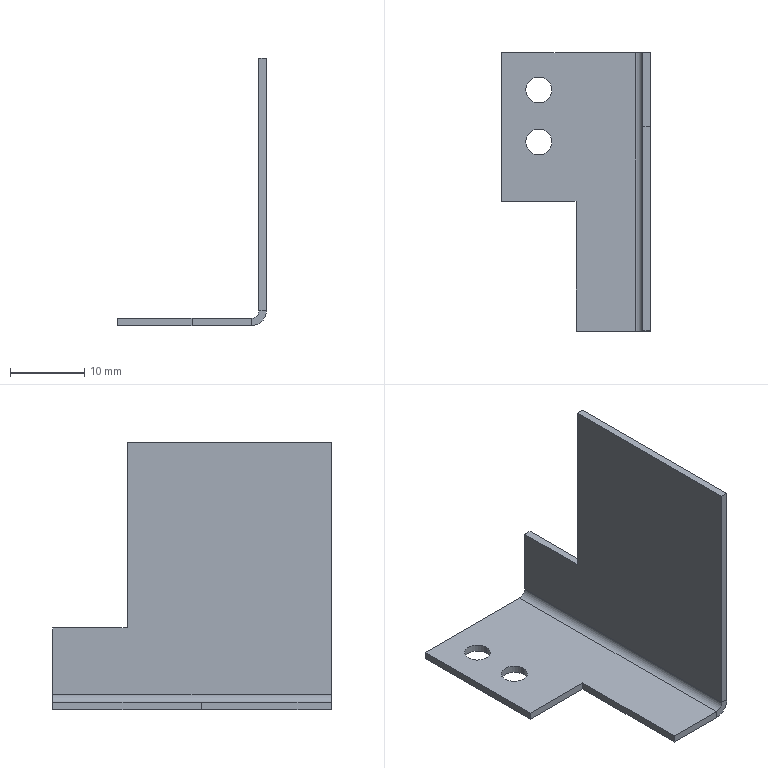Part | STEP file | Proximity switch bracket 3V1.201001 | 1 solid | 22 faces | box 20 x 37.5 x 36 mm | volume 1594 mm3 | plane 16 | cylinder 6 | commonest cylinder face diameters 3.5 x4 2 x1 4 x1
STEP:
#1=CARTESIAN_POINT('',(0.,0.,0.));
#2=DIRECTION('',(0.,0.,1.));
#3=DIRECTION('',(1.,0.,0.));
#4=AXIS2_PLACEMENT_3D('',#1,#2,#3);
#5=CARTESIAN_POINT('',(3.25,13.75,0.));
#6=VERTEX_POINT('',#5);
#7=CARTESIAN_POINT('',(3.25,13.75,-1.));
#8=VERTEX_POINT('',#7);
#9=CARTESIAN_POINT('',(3.25,13.75,0.));
#10=DIRECTION('',(0.,0.,-1.));
#11=VECTOR('',#10,1.);
#12=LINE('',#9,#11);
#13=CARTESIAN_POINT('',(5.,13.75,0.));
#14=DIRECTION('',(0.,0.,-1.));
#15=DIRECTION('',(-1.,0.,0.));
#16=AXIS2_PLACEMENT_3D('',#13,#14,#15);
#17=CYLINDRICAL_SURFACE('',#16,1.75);
#18=CARTESIAN_POINT('',(6.283,0.));
#19=DIRECTION('',(0.,1.));
#20=VECTOR('',#19,1.);
#21=LINE('',#18,#20);
#22=(GEOMETRIC_REPRESENTATION_CONTEXT(2)PARAMETRIC_REPRESENTATION_CONTEXT()REPRESENTATION_CONTEXT('',''));
#23=DEFINITIONAL_REPRESENTATION('',(#21),#22);
#24=PCURVE('',#17,#23);
#25=CARTESIAN_POINT('',(5.,13.75,0.));
#26=DIRECTION('',(0.,0.,-1.));
#27=DIRECTION('',(-1.,0.,0.));
#28=AXIS2_PLACEMENT_3D('',#25,#26,#27);
#29=CYLINDRICAL_SURFACE('',#28,1.75);
#30=CARTESIAN_POINT('',(0.,0.));
#31=DIRECTION('',(0.,1.));
#32=VECTOR('',#31,1.);
#33=LINE('',#30,#32);
#34=(GEOMETRIC_REPRESENTATION_CONTEXT(2)PARAMETRIC_REPRESENTATION_CONTEXT()REPRESENTATION_CONTEXT('',''));
#35=DEFINITIONAL_REPRESENTATION('',(#33),#34);
#36=PCURVE('',#29,#35);
#37=SURFACE_CURVE('',#12,(#24,#36),.PCURVE_S1.);
#38=EDGE_CURVE('',#6,#8,#37,.T.);
#39=ORIENTED_EDGE('',*,*,#38,.T.);
#40=CARTESIAN_POINT('',(6.75,13.75,-1.));
#41=VERTEX_POINT('',#40);
#42=CARTESIAN_POINT('',(5.,13.75,-1.));
#43=DIRECTION('',(0.,0.,-1.));
#44=DIRECTION('',(-1.,0.,0.));
#45=AXIS2_PLACEMENT_3D('',#42,#43,#44);
#46=CIRCLE('',#45,1.75);
#47=CARTESIAN_POINT('',(0.,1.));
#48=DIRECTION('',(1.,0.));
#49=VECTOR('',#48,1.);
#50=LINE('',#47,#49);
#51=(GEOMETRIC_REPRESENTATION_CONTEXT(2)PARAMETRIC_REPRESENTATION_CONTEXT()REPRESENTATION_CONTEXT('',''));
#52=DEFINITIONAL_REPRESENTATION('',(#50),#51);
#53=PCURVE('',#17,#52);
#54=CARTESIAN_POINT('',(0.,18.75,-1.));
#55=DIRECTION('',(0.,0.,-1.));
#56=DIRECTION('',(-1.,0.,0.));
#57=AXIS2_PLACEMENT_3D('',#54,#55,#56);
#58=PLANE('',#57);
#59=CARTESIAN_POINT('',(-5.,-5.));
#60=DIRECTION('',(1.,0.));
#61=AXIS2_PLACEMENT_2D('',#59,#60);
#62=CIRCLE('',#61,1.75);
#63=(GEOMETRIC_REPRESENTATION_CONTEXT(2)PARAMETRIC_REPRESENTATION_CONTEXT()REPRESENTATION_CONTEXT('',''));
#64=DEFINITIONAL_REPRESENTATION('',(#62),#63);
#65=PCURVE('',#58,#64);
#66=SURFACE_CURVE('',#46,(#53,#65),.PCURVE_S1.);
#67=EDGE_CURVE('',#41,#8,#66,.T.);
#68=ORIENTED_EDGE('',*,*,#67,.F.);
#69=CARTESIAN_POINT('',(6.75,13.75,0.));
#70=VERTEX_POINT('',#69);
#71=CARTESIAN_POINT('',(6.75,13.75,0.));
#72=DIRECTION('',(0.,0.,-1.));
#73=VECTOR('',#72,1.);
#74=LINE('',#71,#73);
#75=CARTESIAN_POINT('',(3.142,0.));
#76=DIRECTION('',(0.,1.));
#77=VECTOR('',#76,1.);
#78=LINE('',#75,#77);
#79=(GEOMETRIC_REPRESENTATION_CONTEXT(2)PARAMETRIC_REPRESENTATION_CONTEXT()REPRESENTATION_CONTEXT('',''));
#80=DEFINITIONAL_REPRESENTATION('',(#78),#79);
#81=PCURVE('',#17,#80);
#82=CARTESIAN_POINT('',(3.142,0.));
#83=DIRECTION('',(0.,1.));
#84=VECTOR('',#83,1.);
#85=LINE('',#82,#84);
#86=(GEOMETRIC_REPRESENTATION_CONTEXT(2)PARAMETRIC_REPRESENTATION_CONTEXT()REPRESENTATION_CONTEXT('',''));
#87=DEFINITIONAL_REPRESENTATION('',(#85),#86);
#88=PCURVE('',#29,#87);
#89=SURFACE_CURVE('',#74,(#81,#88),.PCURVE_S1.);
#90=EDGE_CURVE('',#70,#41,#89,.T.);
#91=ORIENTED_EDGE('',*,*,#90,.F.);
#92=CARTESIAN_POINT('',(5.,13.75,0.));
#93=DIRECTION('',(0.,0.,-1.));
#94=DIRECTION('',(-1.,0.,0.));
#95=AXIS2_PLACEMENT_3D('',#92,#93,#94);
#96=CIRCLE('',#95,1.75);
#97=CARTESIAN_POINT('',(0.,0.));
#98=DIRECTION('',(1.,0.));
#99=VECTOR('',#98,1.);
#100=LINE('',#97,#99);
#101=(GEOMETRIC_REPRESENTATION_CONTEXT(2)PARAMETRIC_REPRESENTATION_CONTEXT()REPRESENTATION_CONTEXT('',''));
#102=DEFINITIONAL_REPRESENTATION('',(#100),#101);
#103=PCURVE('',#17,#102);
#104=CARTESIAN_POINT('',(0.,18.75,0.));
#105=DIRECTION('',(0.,0.,-1.));
#106=DIRECTION('',(-1.,0.,0.));
#107=AXIS2_PLACEMENT_3D('',#104,#105,#106);
#108=PLANE('',#107);
#109=CARTESIAN_POINT('',(-5.,-5.));
#110=DIRECTION('',(1.,0.));
#111=AXIS2_PLACEMENT_2D('',#109,#110);
#112=CIRCLE('',#111,1.75);
#113=(GEOMETRIC_REPRESENTATION_CONTEXT(2)PARAMETRIC_REPRESENTATION_CONTEXT()REPRESENTATION_CONTEXT('',''));
#114=DEFINITIONAL_REPRESENTATION('',(#112),#113);
#115=PCURVE('',#108,#114);
#116=SURFACE_CURVE('',#96,(#103,#115),.PCURVE_S1.);
#117=EDGE_CURVE('',#70,#6,#116,.T.);
#118=ORIENTED_EDGE('',*,*,#117,.T.);
#119=EDGE_LOOP('',(#39,#68,#91,#118));
#120=FACE_BOUND('',#119,.F.);
#121=ADVANCED_FACE('',(#120),#17,.F.);
#122=CARTESIAN_POINT('',(3.25,6.75,0.));
#123=VERTEX_POINT('',#122);
#124=CARTESIAN_POINT('',(3.25,6.75,-1.));
#125=VERTEX_POINT('',#124);
#126=CARTESIAN_POINT('',(3.25,6.75,0.));
#127=DIRECTION('',(0.,0.,-1.));
#128=VECTOR('',#127,1.);
#129=LINE('',#126,#128);
#130=CARTESIAN_POINT('',(5.,6.75,0.));
#131=DIRECTION('',(0.,0.,-1.));
#132=DIRECTION('',(-1.,0.,0.));
#133=AXIS2_PLACEMENT_3D('',#130,#131,#132);
#134=CYLINDRICAL_SURFACE('',#133,1.75);
#135=CARTESIAN_POINT('',(6.283,0.));
#136=DIRECTION('',(0.,1.));
#137=VECTOR('',#136,1.);
#138=LINE('',#135,#137);
#139=(GEOMETRIC_REPRESENTATION_CONTEXT(2)PARAMETRIC_REPRESENTATION_CONTEXT()REPRESENTATION_CONTEXT('',''));
#140=DEFINITIONAL_REPRESENTATION('',(#138),#139);
#141=PCURVE('',#134,#140);
#142=CARTESIAN_POINT('',(5.,6.75,0.));
#143=DIRECTION('',(0.,0.,-1.));
#144=DIRECTION('',(-1.,0.,0.));
#145=AXIS2_PLACEMENT_3D('',#142,#143,#144);
#146=CYLINDRICAL_SURFACE('',#145,1.75);
#147=CARTESIAN_POINT('',(0.,0.));
#148=DIRECTION('',(0.,1.));
#149=VECTOR('',#148,1.);
#150=LINE('',#147,#149);
#151=(GEOMETRIC_REPRESENTATION_CONTEXT(2)PARAMETRIC_REPRESENTATION_CONTEXT()REPRESENTATION_CONTEXT('',''));
#152=DEFINITIONAL_REPRESENTATION('',(#150),#151);
#153=PCURVE('',#146,#152);
#154=SURFACE_CURVE('',#129,(#141,#153),.PCURVE_S1.);
#155=EDGE_CURVE('',#123,#125,#154,.T.);
#156=ORIENTED_EDGE('',*,*,#155,.T.);
#157=CARTESIAN_POINT('',(6.75,6.75,-1.));
#158=VERTEX_POINT('',#157);
#159=CARTESIAN_POINT('',(5.,6.75,-1.));
#160=DIRECTION('',(0.,0.,-1.));
#161=DIRECTION('',(1.,0.,0.));
#162=AXIS2_PLACEMENT_3D('',#159,#160,#161);
#163=CIRCLE('',#162,1.75);
#164=CARTESIAN_POINT('',(3.142,1.));
#165=DIRECTION('',(1.,0.));
#166=VECTOR('',#165,1.);
#167=LINE('',#164,#166);
#168=(GEOMETRIC_REPRESENTATION_CONTEXT(2)PARAMETRIC_REPRESENTATION_CONTEXT()REPRESENTATION_CONTEXT('',''));
#169=DEFINITIONAL_REPRESENTATION('',(#167),#168);
#170=PCURVE('',#134,#169);
#171=CARTESIAN_POINT('',(-5.,-12.));
#172=DIRECTION('',(-1.,0.));
#173=AXIS2_PLACEMENT_2D('',#171,#172);
#174=CIRCLE('',#173,1.75);
#175=(GEOMETRIC_REPRESENTATION_CONTEXT(2)PARAMETRIC_REPRESENTATION_CONTEXT()REPRESENTATION_CONTEXT('',''));
#176=DEFINITIONAL_REPRESENTATION('',(#174),#175);
#177=PCURVE('',#58,#176);
#178=SURFACE_CURVE('',#163,(#170,#177),.PCURVE_S1.);
#179=EDGE_CURVE('',#158,#125,#178,.T.);
#180=ORIENTED_EDGE('',*,*,#179,.F.);
#181=CARTESIAN_POINT('',(6.75,6.75,0.));
#182=VERTEX_POINT('',#181);
#183=CARTESIAN_POINT('',(6.75,6.75,0.));
#184=DIRECTION('',(0.,0.,-1.));
#185=VECTOR('',#184,1.);
#186=LINE('',#183,#185);
#187=CARTESIAN_POINT('',(3.142,0.));
#188=DIRECTION('',(0.,1.));
#189=VECTOR('',#188,1.);
#190=LINE('',#187,#189);
#191=(GEOMETRIC_REPRESENTATION_CONTEXT(2)PARAMETRIC_REPRESENTATION_CONTEXT()REPRESENTATION_CONTEXT('',''));
#192=DEFINITIONAL_REPRESENTATION('',(#190),#191);
#193=PCURVE('',#134,#192);
#194=CARTESIAN_POINT('',(3.142,0.));
#195=DIRECTION('',(0.,1.));
#196=VECTOR('',#195,1.);
#197=LINE('',#194,#196);
#198=(GEOMETRIC_REPRESENTATION_CONTEXT(2)PARAMETRIC_REPRESENTATION_CONTEXT()REPRESENTATION_CONTEXT('',''));
#199=DEFINITIONAL_REPRESENTATION('',(#197),#198);
#200=PCURVE('',#146,#199);
#201=SURFACE_CURVE('',#186,(#193,#200),.PCURVE_S1.);
#202=EDGE_CURVE('',#182,#158,#201,.T.);
#203=ORIENTED_EDGE('',*,*,#202,.F.);
#204=CARTESIAN_POINT('',(5.,6.75,0.));
#205=DIRECTION('',(0.,0.,-1.));
#206=DIRECTION('',(1.,0.,0.));
#207=AXIS2_PLACEMENT_3D('',#204,#205,#206);
#208=CIRCLE('',#207,1.75);
#209=CARTESIAN_POINT('',(3.142,0.));
#210=DIRECTION('',(1.,0.));
#211=VECTOR('',#210,1.);
#212=LINE('',#209,#211);
#213=(GEOMETRIC_REPRESENTATION_CONTEXT(2)PARAMETRIC_REPRESENTATION_CONTEXT()REPRESENTATION_CONTEXT('',''));
#214=DEFINITIONAL_REPRESENTATION('',(#212),#213);
#215=PCURVE('',#134,#214);
#216=CARTESIAN_POINT('',(-5.,-12.));
#217=DIRECTION('',(-1.,0.));
#218=AXIS2_PLACEMENT_2D('',#216,#217);
#219=CIRCLE('',#218,1.75);
#220=(GEOMETRIC_REPRESENTATION_CONTEXT(2)PARAMETRIC_REPRESENTATION_CONTEXT()REPRESENTATION_CONTEXT('',''));
#221=DEFINITIONAL_REPRESENTATION('',(#219),#220);
#222=PCURVE('',#108,#221);
#223=SURFACE_CURVE('',#208,(#215,#222),.PCURVE_S1.);
#224=EDGE_CURVE('',#182,#123,#223,.T.);
#225=ORIENTED_EDGE('',*,*,#224,.T.);
#226=EDGE_LOOP('',(#156,#180,#203,#225));
#227=FACE_BOUND('',#226,.F.);
#228=ADVANCED_FACE('',(#227),#134,.F.);
#229=CARTESIAN_POINT('',(5.,6.75,0.));
#230=DIRECTION('',(0.,0.,-1.));
#231=DIRECTION('',(1.,0.,0.));
#232=AXIS2_PLACEMENT_3D('',#229,#230,#231);
#233=CIRCLE('',#232,1.75);
#234=CARTESIAN_POINT('',(-5.,-12.));
#235=DIRECTION('',(-1.,0.));
#236=AXIS2_PLACEMENT_2D('',#234,#235);
#237=CIRCLE('',#236,1.75);
#238=(GEOMETRIC_REPRESENTATION_CONTEXT(2)PARAMETRIC_REPRESENTATION_CONTEXT()REPRESENTATION_CONTEXT('',''));
#239=DEFINITIONAL_REPRESENTATION('',(#237),#238);
#240=PCURVE('',#108,#239);
#241=CARTESIAN_POINT('',(-3.142,0.));
#242=DIRECTION('',(1.,0.));
#243=VECTOR('',#242,1.);
#244=LINE('',#241,#243);
#245=(GEOMETRIC_REPRESENTATION_CONTEXT(2)PARAMETRIC_REPRESENTATION_CONTEXT()REPRESENTATION_CONTEXT('',''));
#246=DEFINITIONAL_REPRESENTATION('',(#244),#245);
#247=PCURVE('',#146,#246);
#248=SURFACE_CURVE('',#233,(#240,#247),.PCURVE_S1.);
#249=EDGE_CURVE('',#123,#182,#248,.T.);
#250=ORIENTED_EDGE('',*,*,#249,.T.);
#251=ORIENTED_EDGE('',*,*,#224,.T.);
#252=EDGE_LOOP('',(#250,#251));
#253=FACE_BOUND('',#252,.T.);
#254=CARTESIAN_POINT('',(5.,13.75,0.));
#255=DIRECTION('',(0.,0.,-1.));
#256=DIRECTION('',(-1.,0.,0.));
#257=AXIS2_PLACEMENT_3D('',#254,#255,#256);
#258=CIRCLE('',#257,1.75);
#259=CARTESIAN_POINT('',(-5.,-5.));
#260=DIRECTION('',(1.,0.));
#261=AXIS2_PLACEMENT_2D('',#259,#260);
#262=CIRCLE('',#261,1.75);
#263=(GEOMETRIC_REPRESENTATION_CONTEXT(2)PARAMETRIC_REPRESENTATION_CONTEXT()REPRESENTATION_CONTEXT('',''));
#264=DEFINITIONAL_REPRESENTATION('',(#262),#263);
#265=PCURVE('',#108,#264);
#266=CARTESIAN_POINT('',(0.,0.));
#267=DIRECTION('',(1.,0.));
#268=VECTOR('',#267,1.);
#269=LINE('',#266,#268);
#270=(GEOMETRIC_REPRESENTATION_CONTEXT(2)PARAMETRIC_REPRESENTATION_CONTEXT()REPRESENTATION_CONTEXT('',''));
#271=DEFINITIONAL_REPRESENTATION('',(#269),#270);
#272=PCURVE('',#29,#271);
#273=SURFACE_CURVE('',#258,(#265,#272),.PCURVE_S1.);
#274=EDGE_CURVE('',#6,#70,#273,.T.);
#275=ORIENTED_EDGE('',*,*,#274,.T.);
#276=ORIENTED_EDGE('',*,*,#117,.T.);
#277=EDGE_LOOP('',(#275,#276));
#278=FACE_BOUND('',#277,.T.);
#279=CARTESIAN_POINT('',(0.,-1.25,0.));
#280=VERTEX_POINT('',#279);
#281=CARTESIAN_POINT('',(10.,-1.25,0.));
#282=VERTEX_POINT('',#281);
#283=CARTESIAN_POINT('',(0.,-1.25,0.));
#284=DIRECTION('',(1.,0.,0.));
#285=VECTOR('',#284,1.);
#286=LINE('',#283,#285);
#287=CARTESIAN_POINT('',(0.,-20.));
#288=DIRECTION('',(-1.,0.));
#289=VECTOR('',#288,1.);
#290=LINE('',#287,#289);
#291=(GEOMETRIC_REPRESENTATION_CONTEXT(2)PARAMETRIC_REPRESENTATION_CONTEXT()REPRESENTATION_CONTEXT('',''));
#292=DEFINITIONAL_REPRESENTATION('',(#290),#291);
#293=PCURVE('',#108,#292);
#294=CARTESIAN_POINT('',(0.,-1.25,9.));
#295=DIRECTION('',(0.,1.,0.));
#296=DIRECTION('',(-1.,0.,0.));
#297=AXIS2_PLACEMENT_3D('',#294,#295,#296);
#298=PLANE('',#297);
#299=CARTESIAN_POINT('',(0.,-9.));
#300=DIRECTION('',(-1.,0.));
#301=VECTOR('',#300,1.);
#302=LINE('',#299,#301);
#303=(GEOMETRIC_REPRESENTATION_CONTEXT(2)PARAMETRIC_REPRESENTATION_CONTEXT()REPRESENTATION_CONTEXT('',''));
#304=DEFINITIONAL_REPRESENTATION('',(#302),#303);
#305=PCURVE('',#298,#304);
#306=SURFACE_CURVE('',#286,(#293,#305),.PCURVE_S1.);
#307=EDGE_CURVE('',#280,#282,#306,.T.);
#308=ORIENTED_EDGE('',*,*,#307,.T.);
#309=CARTESIAN_POINT('',(10.,-18.75,0.));
#310=VERTEX_POINT('',#309);
#311=CARTESIAN_POINT('',(10.,18.75,0.));
#312=DIRECTION('',(0.,-1.,0.));
#313=VECTOR('',#312,1.);
#314=LINE('',#311,#313);
#315=CARTESIAN_POINT('',(-10.,0.));
#316=DIRECTION('',(0.,-1.));
#317=VECTOR('',#316,1.);
#318=LINE('',#315,#317);
#319=(GEOMETRIC_REPRESENTATION_CONTEXT(2)PARAMETRIC_REPRESENTATION_CONTEXT()REPRESENTATION_CONTEXT('',''));
#320=DEFINITIONAL_REPRESENTATION('',(#318),#319);
#321=PCURVE('',#108,#320);
#322=CARTESIAN_POINT('',(10.,-18.75,9.));
#323=DIRECTION('',(1.,0.,0.));
#324=DIRECTION('',(0.,0.,-1.));
#325=AXIS2_PLACEMENT_3D('',#322,#323,#324);
#326=PLANE('',#325);
#327=CARTESIAN_POINT('',(9.,37.5));
#328=DIRECTION('',(0.,-1.));
#329=VECTOR('',#328,1.);
#330=LINE('',#327,#329);
#331=(GEOMETRIC_REPRESENTATION_CONTEXT(2)PARAMETRIC_REPRESENTATION_CONTEXT()REPRESENTATION_CONTEXT('',''));
#332=DEFINITIONAL_REPRESENTATION('',(#330),#331);
#333=PCURVE('',#326,#332);
#334=SURFACE_CURVE('',#314,(#321,#333),.PCURVE_S1.);
#335=EDGE_CURVE('',#282,#310,#334,.T.);
#336=ORIENTED_EDGE('',*,*,#335,.T.);
#337=CARTESIAN_POINT('',(18.,-18.75,0.));
#338=VERTEX_POINT('',#337);
#339=CARTESIAN_POINT('',(0.,-18.75,0.));
#340=DIRECTION('',(1.,0.,0.));
#341=VECTOR('',#340,1.);
#342=LINE('',#339,#341);
#343=CARTESIAN_POINT('',(0.,-37.5));
#344=DIRECTION('',(-1.,0.));
#345=VECTOR('',#344,1.);
#346=LINE('',#343,#345);
#347=(GEOMETRIC_REPRESENTATION_CONTEXT(2)PARAMETRIC_REPRESENTATION_CONTEXT()REPRESENTATION_CONTEXT('',''));
#348=DEFINITIONAL_REPRESENTATION('',(#346),#347);
#349=PCURVE('',#108,#348);
#350=CARTESIAN_POINT('',(0.,-18.75,0.));
#351=DIRECTION('',(0.,-1.,0.));
#352=DIRECTION('',(-1.,0.,0.));
#353=AXIS2_PLACEMENT_3D('',#350,#351,#352);
#354=PLANE('',#353);
#355=CARTESIAN_POINT('',(0.,0.));
#356=DIRECTION('',(-1.,0.));
#357=VECTOR('',#356,1.);
#358=LINE('',#355,#357);
#359=(GEOMETRIC_REPRESENTATION_CONTEXT(2)PARAMETRIC_REPRESENTATION_CONTEXT()REPRESENTATION_CONTEXT('',''));
#360=DEFINITIONAL_REPRESENTATION('',(#358),#359);
#361=PCURVE('',#354,#360);
#362=SURFACE_CURVE('',#342,(#349,#361),.PCURVE_S1.);
#363=EDGE_CURVE('',#310,#338,#362,.T.);
#364=ORIENTED_EDGE('',*,*,#363,.T.);
#365=CARTESIAN_POINT('',(18.,18.75,0.));
#366=VERTEX_POINT('',#365);
#367=CARTESIAN_POINT('',(18.,18.75,0.));
#368=DIRECTION('',(0.,-1.,0.));
#369=VECTOR('',#368,1.);
#370=LINE('',#367,#369);
#371=CARTESIAN_POINT('',(-18.,0.));
#372=DIRECTION('',(0.,-1.));
#373=VECTOR('',#372,1.);
#374=LINE('',#371,#373);
#375=(GEOMETRIC_REPRESENTATION_CONTEXT(2)PARAMETRIC_REPRESENTATION_CONTEXT()REPRESENTATION_CONTEXT('',''));
#376=DEFINITIONAL_REPRESENTATION('',(#374),#375);
#377=PCURVE('',#108,#376);
#378=CARTESIAN_POINT('',(18.,18.75,1.));
#379=DIRECTION('',(0.,1.,0.));
#380=DIRECTION('',(1.,0.,0.));
#381=AXIS2_PLACEMENT_3D('',#378,#379,#380);
#382=CYLINDRICAL_SURFACE('',#381,1.);
#383=CARTESIAN_POINT('',(1.571,0.));
#384=DIRECTION('',(0.,-1.));
#385=VECTOR('',#384,1.);
#386=LINE('',#383,#385);
#387=(GEOMETRIC_REPRESENTATION_CONTEXT(2)PARAMETRIC_REPRESENTATION_CONTEXT()REPRESENTATION_CONTEXT('',''));
#388=DEFINITIONAL_REPRESENTATION('',(#386),#387);
#389=PCURVE('',#382,#388);
#390=SURFACE_CURVE('',#370,(#377,#389),.PCURVE_S1.);
#391=EDGE_CURVE('',#366,#338,#390,.T.);
#392=ORIENTED_EDGE('',*,*,#391,.F.);
#393=CARTESIAN_POINT('',(0.,18.75,0.));
#394=VERTEX_POINT('',#393);
#395=CARTESIAN_POINT('',(0.,18.75,0.));
#396=DIRECTION('',(1.,0.,0.));
#397=VECTOR('',#396,1.);
#398=LINE('',#395,#397);
#399=CARTESIAN_POINT('',(0.,0.));
#400=DIRECTION('',(-1.,0.));
#401=VECTOR('',#400,1.);
#402=LINE('',#399,#401);
#403=(GEOMETRIC_REPRESENTATION_CONTEXT(2)PARAMETRIC_REPRESENTATION_CONTEXT()REPRESENTATION_CONTEXT('',''));
#404=DEFINITIONAL_REPRESENTATION('',(#402),#403);
#405=PCURVE('',#108,#404);
#406=CARTESIAN_POINT('',(0.,18.75,0.));
#407=DIRECTION('',(0.,-1.,0.));
#408=DIRECTION('',(-1.,0.,0.));
#409=AXIS2_PLACEMENT_3D('',#406,#407,#408);
#410=PLANE('',#409);
#411=CARTESIAN_POINT('',(0.,0.));
#412=DIRECTION('',(-1.,0.));
#413=VECTOR('',#412,1.);
#414=LINE('',#411,#413);
#415=(GEOMETRIC_REPRESENTATION_CONTEXT(2)PARAMETRIC_REPRESENTATION_CONTEXT()REPRESENTATION_CONTEXT('',''));
#416=DEFINITIONAL_REPRESENTATION('',(#414),#415);
#417=PCURVE('',#410,#416);
#418=SURFACE_CURVE('',#398,(#405,#417),.PCURVE_S1.);
#419=EDGE_CURVE('',#394,#366,#418,.T.);
#420=ORIENTED_EDGE('',*,*,#419,.F.);
#421=CARTESIAN_POINT('',(0.,18.75,0.));
#422=DIRECTION('',(0.,-1.,0.));
#423=VECTOR('',#422,1.);
#424=LINE('',#421,#423);
#425=CARTESIAN_POINT('',(0.,0.));
#426=DIRECTION('',(0.,-1.));
#427=VECTOR('',#426,1.);
#428=LINE('',#425,#427);
#429=(GEOMETRIC_REPRESENTATION_CONTEXT(2)PARAMETRIC_REPRESENTATION_CONTEXT()REPRESENTATION_CONTEXT('',''));
#430=DEFINITIONAL_REPRESENTATION('',(#428),#429);
#431=PCURVE('',#108,#430);
#432=CARTESIAN_POINT('',(0.,18.75,0.));
#433=DIRECTION('',(-1.,0.,0.));
#434=DIRECTION('',(0.,0.,1.));
#435=AXIS2_PLACEMENT_3D('',#432,#433,#434);
#436=PLANE('',#435);
#437=CARTESIAN_POINT('',(0.,0.));
#438=DIRECTION('',(0.,-1.));
#439=VECTOR('',#438,1.);
#440=LINE('',#437,#439);
#441=(GEOMETRIC_REPRESENTATION_CONTEXT(2)PARAMETRIC_REPRESENTATION_CONTEXT()REPRESENTATION_CONTEXT('',''));
#442=DEFINITIONAL_REPRESENTATION('',(#440),#441);
#443=PCURVE('',#436,#442);
#444=SURFACE_CURVE('',#424,(#431,#443),.PCURVE_S1.);
#445=EDGE_CURVE('',#394,#280,#444,.T.);
#446=ORIENTED_EDGE('',*,*,#445,.T.);
#447=EDGE_LOOP('',(#308,#336,#364,#392,#420,#446));
#448=FACE_BOUND('',#447,.T.);
#449=ADVANCED_FACE('',(#253,#278,#448),#108,.F.);
#450=CARTESIAN_POINT('',(10.,-1.25,-1.));
#451=VERTEX_POINT('',#450);
#452=CARTESIAN_POINT('',(10.,-18.75,-1.));
#453=VERTEX_POINT('',#452);
#454=CARTESIAN_POINT('',(10.,-18.75,-1.));
#455=DIRECTION('',(0.,-1.,0.));
#456=VECTOR('',#455,1.);
#457=LINE('',#454,#456);
#458=CARTESIAN_POINT('',(-10.,-37.5));
#459=DIRECTION('',(0.,-1.));
#460=VECTOR('',#459,1.);
#461=LINE('',#458,#460);
#462=(GEOMETRIC_REPRESENTATION_CONTEXT(2)PARAMETRIC_REPRESENTATION_CONTEXT()REPRESENTATION_CONTEXT('',''));
#463=DEFINITIONAL_REPRESENTATION('',(#461),#462);
#464=PCURVE('',#58,#463);
#465=CARTESIAN_POINT('',(10.,0.));
#466=DIRECTION('',(0.,-1.));
#467=VECTOR('',#466,1.);
#468=LINE('',#465,#467);
#469=(GEOMETRIC_REPRESENTATION_CONTEXT(2)PARAMETRIC_REPRESENTATION_CONTEXT()REPRESENTATION_CONTEXT('',''));
#470=DEFINITIONAL_REPRESENTATION('',(#468),#469);
#471=PCURVE('',#326,#470);
#472=SURFACE_CURVE('',#457,(#464,#471),.PCURVE_S1.);
#473=EDGE_CURVE('',#451,#453,#472,.T.);
#474=ORIENTED_EDGE('',*,*,#473,.F.);
#475=CARTESIAN_POINT('',(0.,-1.25,-1.));
#476=VERTEX_POINT('',#475);
#477=CARTESIAN_POINT('',(0.,-1.25,-1.));
#478=DIRECTION('',(1.,0.,0.));
#479=VECTOR('',#478,1.);
#480=LINE('',#477,#479);
#481=CARTESIAN_POINT('',(0.,-20.));
#482=DIRECTION('',(-1.,0.));
#483=VECTOR('',#482,1.);
#484=LINE('',#481,#483);
#485=(GEOMETRIC_REPRESENTATION_CONTEXT(2)PARAMETRIC_REPRESENTATION_CONTEXT()REPRESENTATION_CONTEXT('',''));
#486=DEFINITIONAL_REPRESENTATION('',(#484),#485);
#487=PCURVE('',#58,#486);
#488=CARTESIAN_POINT('',(0.,-10.));
#489=DIRECTION('',(-1.,0.));
#490=VECTOR('',#489,1.);
#491=LINE('',#488,#490);
#492=(GEOMETRIC_REPRESENTATION_CONTEXT(2)PARAMETRIC_REPRESENTATION_CONTEXT()REPRESENTATION_CONTEXT('',''));
#493=DEFINITIONAL_REPRESENTATION('',(#491),#492);
#494=PCURVE('',#298,#493);
#495=SURFACE_CURVE('',#480,(#487,#494),.PCURVE_S1.);
#496=EDGE_CURVE('',#476,#451,#495,.T.);
#497=ORIENTED_EDGE('',*,*,#496,.F.);
#498=CARTESIAN_POINT('',(0.,18.75,-1.));
#499=VERTEX_POINT('',#498);
#500=CARTESIAN_POINT('',(0.,18.75,-1.));
#501=DIRECTION('',(0.,-1.,0.));
#502=VECTOR('',#501,1.);
#503=LINE('',#500,#502);
#504=CARTESIAN_POINT('',(0.,0.));
#505=DIRECTION('',(0.,-1.));
#506=VECTOR('',#505,1.);
#507=LINE('',#504,#506);
#508=(GEOMETRIC_REPRESENTATION_CONTEXT(2)PARAMETRIC_REPRESENTATION_CONTEXT()REPRESENTATION_CONTEXT('',''));
#509=DEFINITIONAL_REPRESENTATION('',(#507),#508);
#510=PCURVE('',#58,#509);
#511=CARTESIAN_POINT('',(-1.,0.));
#512=DIRECTION('',(0.,-1.));
#513=VECTOR('',#512,1.);
#514=LINE('',#511,#513);
#515=(GEOMETRIC_REPRESENTATION_CONTEXT(2)PARAMETRIC_REPRESENTATION_CONTEXT()REPRESENTATION_CONTEXT('',''));
#516=DEFINITIONAL_REPRESENTATION('',(#514),#515);
#517=PCURVE('',#436,#516);
#518=SURFACE_CURVE('',#503,(#510,#517),.PCURVE_S1.);
#519=EDGE_CURVE('',#499,#476,#518,.T.);
#520=ORIENTED_EDGE('',*,*,#519,.F.);
#521=CARTESIAN_POINT('',(18.,18.75,-1.));
#522=VERTEX_POINT('',#521);
#523=CARTESIAN_POINT('',(0.,18.75,-1.));
#524=DIRECTION('',(1.,0.,0.));
#525=VECTOR('',#524,1.);
#526=LINE('',#523,#525);
#527=CARTESIAN_POINT('',(0.,0.));
#528=DIRECTION('',(-1.,0.));
#529=VECTOR('',#528,1.);
#530=LINE('',#527,#529);
#531=(GEOMETRIC_REPRESENTATION_CONTEXT(2)PARAMETRIC_REPRESENTATION_CONTEXT()REPRESENTATION_CONTEXT('',''));
#532=DEFINITIONAL_REPRESENTATION('',(#530),#531);
#533=PCURVE('',#58,#532);
#534=CARTESIAN_POINT('',(0.,1.));
#535=DIRECTION('',(-1.,0.));
#536=VECTOR('',#535,1.);
#537=LINE('',#534,#536);
#538=(GEOMETRIC_REPRESENTATION_CONTEXT(2)PARAMETRIC_REPRESENTATION_CONTEXT()REPRESENTATION_CONTEXT('',''));
#539=DEFINITIONAL_REPRESENTATION('',(#537),#538);
#540=PCURVE('',#410,#539);
#541=SURFACE_CURVE('',#526,(#533,#540),.PCURVE_S1.);
#542=EDGE_CURVE('',#499,#522,#541,.T.);
#543=ORIENTED_EDGE('',*,*,#542,.T.);
#544=CARTESIAN_POINT('',(18.,-18.75,-1.));
#545=VERTEX_POINT('',#544);
#546=CARTESIAN_POINT('',(18.,18.75,-1.));
#547=DIRECTION('',(0.,-1.,0.));
#548=VECTOR('',#547,1.);
#549=LINE('',#546,#548);
#550=CARTESIAN_POINT('',(-18.,0.));
#551=DIRECTION('',(0.,-1.));
#552=VECTOR('',#551,1.);
#553=LINE('',#550,#552);
#554=(GEOMETRIC_REPRESENTATION_CONTEXT(2)PARAMETRIC_REPRESENTATION_CONTEXT()REPRESENTATION_CONTEXT('',''));
#555=DEFINITIONAL_REPRESENTATION('',(#553),#554);
#556=PCURVE('',#58,#555);
#557=CARTESIAN_POINT('',(18.,18.75,1.));
#558=DIRECTION('',(0.,1.,0.));
#559=DIRECTION('',(1.,0.,0.));
#560=AXIS2_PLACEMENT_3D('',#557,#558,#559);
#561=CYLINDRICAL_SURFACE('',#560,2.);
#562=CARTESIAN_POINT('',(1.571,0.));
#563=DIRECTION('',(0.,-1.));
#564=VECTOR('',#563,1.);
#565=LINE('',#562,#564);
#566=(GEOMETRIC_REPRESENTATION_CONTEXT(2)PARAMETRIC_REPRESENTATION_CONTEXT()REPRESENTATION_CONTEXT('',''));
#567=DEFINITIONAL_REPRESENTATION('',(#565),#566);
#568=PCURVE('',#561,#567);
#569=SURFACE_CURVE('',#549,(#556,#568),.PCURVE_S1.);
#570=EDGE_CURVE('',#522,#545,#569,.T.);
#571=ORIENTED_EDGE('',*,*,#570,.T.);
#572=CARTESIAN_POINT('',(0.,-18.75,-1.));
#573=DIRECTION('',(1.,0.,0.));
#574=VECTOR('',#573,1.);
#575=LINE('',#572,#574);
#576=CARTESIAN_POINT('',(0.,-37.5));
#577=DIRECTION('',(-1.,0.));
#578=VECTOR('',#577,1.);
#579=LINE('',#576,#578);
#580=(GEOMETRIC_REPRESENTATION_CONTEXT(2)PARAMETRIC_REPRESENTATION_CONTEXT()REPRESENTATION_CONTEXT('',''));
#581=DEFINITIONAL_REPRESENTATION('',(#579),#580);
#582=PCURVE('',#58,#581);
#583=CARTESIAN_POINT('',(0.,1.));
#584=DIRECTION('',(-1.,0.));
#585=VECTOR('',#584,1.);
#586=LINE('',#583,#585);
#587=(GEOMETRIC_REPRESENTATION_CONTEXT(2)PARAMETRIC_REPRESENTATION_CONTEXT()REPRESENTATION_CONTEXT('',''));
#588=DEFINITIONAL_REPRESENTATION('',(#586),#587);
#589=PCURVE('',#354,#588);
#590=SURFACE_CURVE('',#575,(#582,#589),.PCURVE_S1.);
#591=EDGE_CURVE('',#453,#545,#590,.T.);
#592=ORIENTED_EDGE('',*,*,#591,.F.);
#593=EDGE_LOOP('',(#474,#497,#520,#543,#571,#592));
#594=FACE_BOUND('',#593,.T.);
#595=CARTESIAN_POINT('',(5.,13.75,-1.));
#596=DIRECTION('',(0.,0.,-1.));
#597=DIRECTION('',(-1.,0.,0.));
#598=AXIS2_PLACEMENT_3D('',#595,#596,#597);
#599=CIRCLE('',#598,1.75);
#600=CARTESIAN_POINT('',(-5.,-5.));
#601=DIRECTION('',(1.,0.));
#602=AXIS2_PLACEMENT_2D('',#600,#601);
#603=CIRCLE('',#602,1.75);
#604=(GEOMETRIC_REPRESENTATION_CONTEXT(2)PARAMETRIC_REPRESENTATION_CONTEXT()REPRESENTATION_CONTEXT('',''));
#605=DEFINITIONAL_REPRESENTATION('',(#603),#604);
#606=PCURVE('',#58,#605);
#607=CARTESIAN_POINT('',(0.,1.));
#608=DIRECTION('',(1.,0.));
#609=VECTOR('',#608,1.);
#610=LINE('',#607,#609);
#611=(GEOMETRIC_REPRESENTATION_CONTEXT(2)PARAMETRIC_REPRESENTATION_CONTEXT()REPRESENTATION_CONTEXT('',''));
#612=DEFINITIONAL_REPRESENTATION('',(#610),#611);
#613=PCURVE('',#29,#612);
#614=SURFACE_CURVE('',#599,(#606,#613),.PCURVE_S1.);
#615=EDGE_CURVE('',#8,#41,#614,.T.);
#616=ORIENTED_EDGE('',*,*,#615,.F.);
#617=ORIENTED_EDGE('',*,*,#67,.F.);
#618=EDGE_LOOP('',(#616,#617));
#619=FACE_BOUND('',#618,.T.);
#620=CARTESIAN_POINT('',(5.,6.75,-1.));
#621=DIRECTION('',(0.,0.,-1.));
#622=DIRECTION('',(1.,0.,0.));
#623=AXIS2_PLACEMENT_3D('',#620,#621,#622);
#624=CIRCLE('',#623,1.75);
#625=CARTESIAN_POINT('',(-5.,-12.));
#626=DIRECTION('',(-1.,0.));
#627=AXIS2_PLACEMENT_2D('',#625,#626);
#628=CIRCLE('',#627,1.75);
#629=(GEOMETRIC_REPRESENTATION_CONTEXT(2)PARAMETRIC_REPRESENTATION_CONTEXT()REPRESENTATION_CONTEXT('',''));
#630=DEFINITIONAL_REPRESENTATION('',(#628),#629);
#631=PCURVE('',#58,#630);
#632=CARTESIAN_POINT('',(-3.142,1.));
#633=DIRECTION('',(1.,0.));
#634=VECTOR('',#633,1.);
#635=LINE('',#632,#634);
#636=(GEOMETRIC_REPRESENTATION_CONTEXT(2)PARAMETRIC_REPRESENTATION_CONTEXT()REPRESENTATION_CONTEXT('',''));
#637=DEFINITIONAL_REPRESENTATION('',(#635),#636);
#638=PCURVE('',#146,#637);
#639=SURFACE_CURVE('',#624,(#631,#638),.PCURVE_S1.);
#640=EDGE_CURVE('',#125,#158,#639,.T.);
#641=ORIENTED_EDGE('',*,*,#640,.F.);
#642=ORIENTED_EDGE('',*,*,#179,.F.);
#643=EDGE_LOOP('',(#641,#642));
#644=FACE_BOUND('',#643,.T.);
#645=ADVANCED_FACE('',(#594,#619,#644),#58,.T.);
#646=CARTESIAN_POINT('',(18.,18.75,0.));
#647=DIRECTION('',(0.,0.,-1.));
#648=VECTOR('',#647,1.);
#649=LINE('',#646,#648);
#650=CARTESIAN_POINT('',(-18.,0.));
#651=DIRECTION('',(0.,1.));
#652=VECTOR('',#651,1.);
#653=LINE('',#650,#652);
#654=(GEOMETRIC_REPRESENTATION_CONTEXT(2)PARAMETRIC_REPRESENTATION_CONTEXT()REPRESENTATION_CONTEXT('',''));
#655=DEFINITIONAL_REPRESENTATION('',(#653),#654);
#656=PCURVE('',#410,#655);
#657=CARTESIAN_POINT('',(18.,18.75,1.));
#658=DIRECTION('',(0.,-1.,0.));
#659=DIRECTION('',(0.,0.,-1.));
#660=AXIS2_PLACEMENT_3D('',#657,#658,#659);
#661=PLANE('',#660);
#662=CARTESIAN_POINT('',(1.,0.));
#663=DIRECTION('',(1.,0.));
#664=VECTOR('',#663,1.);
#665=LINE('',#662,#664);
#666=(GEOMETRIC_REPRESENTATION_CONTEXT(2)PARAMETRIC_REPRESENTATION_CONTEXT()REPRESENTATION_CONTEXT('',''));
#667=DEFINITIONAL_REPRESENTATION('',(#665),#666);
#668=PCURVE('',#661,#667);
#669=SURFACE_CURVE('',#649,(#656,#668),.PCURVE_S1.);
#670=EDGE_CURVE('',#366,#522,#669,.T.);
#671=ORIENTED_EDGE('',*,*,#670,.T.);
#672=ORIENTED_EDGE('',*,*,#542,.F.);
#673=CARTESIAN_POINT('',(0.,18.75,0.));
#674=DIRECTION('',(0.,0.,-1.));
#675=VECTOR('',#674,1.);
#676=LINE('',#673,#675);
#677=CARTESIAN_POINT('',(0.,0.));
#678=DIRECTION('',(0.,1.));
#679=VECTOR('',#678,1.);
#680=LINE('',#677,#679);
#681=(GEOMETRIC_REPRESENTATION_CONTEXT(2)PARAMETRIC_REPRESENTATION_CONTEXT()REPRESENTATION_CONTEXT('',''));
#682=DEFINITIONAL_REPRESENTATION('',(#680),#681);
#683=PCURVE('',#410,#682);
#684=CARTESIAN_POINT('',(0.,0.));
#685=DIRECTION('',(-1.,0.));
#686=VECTOR('',#685,1.);
#687=LINE('',#684,#686);
#688=(GEOMETRIC_REPRESENTATION_CONTEXT(2)PARAMETRIC_REPRESENTATION_CONTEXT()REPRESENTATION_CONTEXT('',''));
#689=DEFINITIONAL_REPRESENTATION('',(#687),#688);
#690=PCURVE('',#436,#689);
#691=SURFACE_CURVE('',#676,(#683,#690),.PCURVE_S1.);
#692=EDGE_CURVE('',#394,#499,#691,.T.);
#693=ORIENTED_EDGE('',*,*,#692,.F.);
#694=ORIENTED_EDGE('',*,*,#419,.T.);
#695=EDGE_LOOP('',(#671,#672,#693,#694));
#696=FACE_BOUND('',#695,.T.);
#697=ADVANCED_FACE('',(#696),#410,.F.);
#698=CARTESIAN_POINT('',(0.,-1.25,9.));
#699=DIRECTION('',(0.,0.,-1.));
#700=VECTOR('',#699,1.);
#701=LINE('',#698,#700);
#702=CARTESIAN_POINT('',(9.,-20.));
#703=DIRECTION('',(-1.,0.));
#704=VECTOR('',#703,1.);
#705=LINE('',#702,#704);
#706=(GEOMETRIC_REPRESENTATION_CONTEXT(2)PARAMETRIC_REPRESENTATION_CONTEXT()REPRESENTATION_CONTEXT('',''));
#707=DEFINITIONAL_REPRESENTATION('',(#705),#706);
#708=PCURVE('',#436,#707);
#709=CARTESIAN_POINT('',(0.,0.));
#710=DIRECTION('',(0.,-1.));
#711=VECTOR('',#710,1.);
#712=LINE('',#709,#711);
#713=(GEOMETRIC_REPRESENTATION_CONTEXT(2)PARAMETRIC_REPRESENTATION_CONTEXT()REPRESENTATION_CONTEXT('',''));
#714=DEFINITIONAL_REPRESENTATION('',(#712),#713);
#715=PCURVE('',#298,#714);
#716=SURFACE_CURVE('',#701,(#708,#715),.PCURVE_S1.);
#717=EDGE_CURVE('',#280,#476,#716,.T.);
#718=ORIENTED_EDGE('',*,*,#717,.F.);
#719=ORIENTED_EDGE('',*,*,#445,.F.);
#720=ORIENTED_EDGE('',*,*,#692,.T.);
#721=ORIENTED_EDGE('',*,*,#519,.T.);
#722=EDGE_LOOP('',(#718,#719,#720,#721));
#723=FACE_BOUND('',#722,.T.);
#724=ADVANCED_FACE('',(#723),#436,.T.);
#725=CARTESIAN_POINT('',(10.,-18.75,0.));
#726=DIRECTION('',(0.,0.,1.));
#727=VECTOR('',#726,1.);
#728=LINE('',#725,#727);
#729=CARTESIAN_POINT('',(-10.,0.));
#730=DIRECTION('',(0.,-1.));
#731=VECTOR('',#730,1.);
#732=LINE('',#729,#731);
#733=(GEOMETRIC_REPRESENTATION_CONTEXT(2)PARAMETRIC_REPRESENTATION_CONTEXT()REPRESENTATION_CONTEXT('',''));
#734=DEFINITIONAL_REPRESENTATION('',(#732),#733);
#735=PCURVE('',#354,#734);
#736=CARTESIAN_POINT('',(9.,0.));
#737=DIRECTION('',(-1.,0.));
#738=VECTOR('',#737,1.);
#739=LINE('',#736,#738);
#740=(GEOMETRIC_REPRESENTATION_CONTEXT(2)PARAMETRIC_REPRESENTATION_CONTEXT()REPRESENTATION_CONTEXT('',''));
#741=DEFINITIONAL_REPRESENTATION('',(#739),#740);
#742=PCURVE('',#326,#741);
#743=SURFACE_CURVE('',#728,(#735,#742),.PCURVE_S1.);
#744=EDGE_CURVE('',#453,#310,#743,.T.);
#745=ORIENTED_EDGE('',*,*,#744,.F.);
#746=ORIENTED_EDGE('',*,*,#591,.T.);
#747=CARTESIAN_POINT('',(18.,-18.75,0.));
#748=DIRECTION('',(0.,0.,-1.));
#749=VECTOR('',#748,1.);
#750=LINE('',#747,#749);
#751=CARTESIAN_POINT('',(-18.,0.));
#752=DIRECTION('',(0.,1.));
#753=VECTOR('',#752,1.);
#754=LINE('',#751,#753);
#755=(GEOMETRIC_REPRESENTATION_CONTEXT(2)PARAMETRIC_REPRESENTATION_CONTEXT()REPRESENTATION_CONTEXT('',''));
#756=DEFINITIONAL_REPRESENTATION('',(#754),#755);
#757=PCURVE('',#354,#756);
#758=CARTESIAN_POINT('',(18.,-18.75,1.));
#759=DIRECTION('',(0.,-1.,0.));
#760=DIRECTION('',(0.,0.,-1.));
#761=AXIS2_PLACEMENT_3D('',#758,#759,#760);
#762=PLANE('',#761);
#763=CARTESIAN_POINT('',(1.,0.));
#764=DIRECTION('',(1.,0.));
#765=VECTOR('',#764,1.);
#766=LINE('',#763,#765);
#767=(GEOMETRIC_REPRESENTATION_CONTEXT(2)PARAMETRIC_REPRESENTATION_CONTEXT()REPRESENTATION_CONTEXT('',''));
#768=DEFINITIONAL_REPRESENTATION('',(#766),#767);
#769=PCURVE('',#762,#768);
#770=SURFACE_CURVE('',#750,(#757,#769),.PCURVE_S1.);
#771=EDGE_CURVE('',#338,#545,#770,.T.);
#772=ORIENTED_EDGE('',*,*,#771,.F.);
#773=ORIENTED_EDGE('',*,*,#363,.F.);
#774=EDGE_LOOP('',(#745,#746,#772,#773));
#775=FACE_BOUND('',#774,.T.);
#776=ADVANCED_FACE('',(#775),#354,.T.);
#777=ORIENTED_EDGE('',*,*,#640,.F.);
#778=ORIENTED_EDGE('',*,*,#155,.F.);
#779=ORIENTED_EDGE('',*,*,#249,.T.);
#780=ORIENTED_EDGE('',*,*,#202,.T.);
#781=EDGE_LOOP('',(#777,#778,#779,#780));
#782=FACE_BOUND('',#781,.F.);
#783=ADVANCED_FACE('',(#782),#146,.F.);
#784=ORIENTED_EDGE('',*,*,#615,.F.);
#785=ORIENTED_EDGE('',*,*,#38,.F.);
#786=ORIENTED_EDGE('',*,*,#274,.T.);
#787=ORIENTED_EDGE('',*,*,#90,.T.);
#788=EDGE_LOOP('',(#784,#785,#786,#787));
#789=FACE_BOUND('',#788,.F.);
#790=ADVANCED_FACE('',(#789),#29,.F.);
#791=CARTESIAN_POINT('',(19.,-18.75,1.));
#792=VERTEX_POINT('',#791);
#793=CARTESIAN_POINT('',(20.,-18.75,1.));
#794=VERTEX_POINT('',#793);
#795=CARTESIAN_POINT('',(20.,-18.75,1.));
#796=DIRECTION('',(1.,0.,0.));
#797=VECTOR('',#796,1.);
#798=LINE('',#795,#797);
#799=CARTESIAN_POINT('',(0.,2.));
#800=DIRECTION('',(0.,1.));
#801=VECTOR('',#800,1.);
#802=LINE('',#799,#801);
#803=(GEOMETRIC_REPRESENTATION_CONTEXT(2)PARAMETRIC_REPRESENTATION_CONTEXT()REPRESENTATION_CONTEXT('',''));
#804=DEFINITIONAL_REPRESENTATION('',(#802),#803);
#805=PCURVE('',#762,#804);
#806=CARTESIAN_POINT('',(20.,-18.75,35.));
#807=DIRECTION('',(0.,-1.,0.));
#808=DIRECTION('',(0.,0.,-1.));
#809=AXIS2_PLACEMENT_3D('',#806,#807,#808);
#810=PLANE('',#809);
#811=CARTESIAN_POINT('',(34.,0.));
#812=DIRECTION('',(0.,1.));
#813=VECTOR('',#812,1.);
#814=LINE('',#811,#813);
#815=(GEOMETRIC_REPRESENTATION_CONTEXT(2)PARAMETRIC_REPRESENTATION_CONTEXT()REPRESENTATION_CONTEXT('',''));
#816=DEFINITIONAL_REPRESENTATION('',(#814),#815);
#817=PCURVE('',#810,#816);
#818=SURFACE_CURVE('',#798,(#805,#817),.PCURVE_S1.);
#819=EDGE_CURVE('',#792,#794,#818,.T.);
#820=ORIENTED_EDGE('',*,*,#819,.F.);
#821=CARTESIAN_POINT('',(18.,-18.75,1.));
#822=DIRECTION('',(0.,-1.,0.));
#823=DIRECTION('',(0.,0.,1.));
#824=AXIS2_PLACEMENT_3D('',#821,#822,#823);
#825=CIRCLE('',#824,1.);
#826=CARTESIAN_POINT('',(0.,0.));
#827=DIRECTION('',(-1.,0.));
#828=AXIS2_PLACEMENT_2D('',#826,#827);
#829=CIRCLE('',#828,1.);
#830=(GEOMETRIC_REPRESENTATION_CONTEXT(2)PARAMETRIC_REPRESENTATION_CONTEXT()REPRESENTATION_CONTEXT('',''));
#831=DEFINITIONAL_REPRESENTATION('',(#829),#830);
#832=PCURVE('',#762,#831);
#833=CARTESIAN_POINT('',(4.712,-37.5));
#834=DIRECTION('',(-1.,0.));
#835=VECTOR('',#834,1.);
#836=LINE('',#833,#835);
#837=(GEOMETRIC_REPRESENTATION_CONTEXT(2)PARAMETRIC_REPRESENTATION_CONTEXT()REPRESENTATION_CONTEXT('',''));
#838=DEFINITIONAL_REPRESENTATION('',(#836),#837);
#839=PCURVE('',#382,#838);
#840=SURFACE_CURVE('',#825,(#832,#839),.PCURVE_S1.);
#841=EDGE_CURVE('',#338,#792,#840,.T.);
#842=ORIENTED_EDGE('',*,*,#841,.F.);
#843=ORIENTED_EDGE('',*,*,#771,.T.);
#844=CARTESIAN_POINT('',(18.,-18.75,1.));
#845=DIRECTION('',(0.,-1.,0.));
#846=DIRECTION('',(0.,0.,1.));
#847=AXIS2_PLACEMENT_3D('',#844,#845,#846);
#848=CIRCLE('',#847,2.);
#849=CARTESIAN_POINT('',(0.,0.));
#850=DIRECTION('',(-1.,0.));
#851=AXIS2_PLACEMENT_2D('',#849,#850);
#852=CIRCLE('',#851,2.);
#853=(GEOMETRIC_REPRESENTATION_CONTEXT(2)PARAMETRIC_REPRESENTATION_CONTEXT()REPRESENTATION_CONTEXT('',''));
#854=DEFINITIONAL_REPRESENTATION('',(#852),#853);
#855=PCURVE('',#762,#854);
#856=CARTESIAN_POINT('',(4.712,-37.5));
#857=DIRECTION('',(-1.,0.));
#858=VECTOR('',#857,1.);
#859=LINE('',#856,#858);
#860=(GEOMETRIC_REPRESENTATION_CONTEXT(2)PARAMETRIC_REPRESENTATION_CONTEXT()REPRESENTATION_CONTEXT('',''));
#861=DEFINITIONAL_REPRESENTATION('',(#859),#860);
#862=PCURVE('',#561,#861);
#863=SURFACE_CURVE('',#848,(#855,#862),.PCURVE_S1.);
#864=EDGE_CURVE('',#545,#794,#863,.T.);
#865=ORIENTED_EDGE('',*,*,#864,.T.);
#866=EDGE_LOOP('',(#820,#842,#843,#865));
#867=FACE_BOUND('',#866,.T.);
#868=ADVANCED_FACE('',(#867),#762,.T.);
#869=CARTESIAN_POINT('',(19.,18.75,1.));
#870=VERTEX_POINT('',#869);
#871=CARTESIAN_POINT('',(18.,18.75,1.));
#872=DIRECTION('',(0.,1.,0.));
#873=DIRECTION('',(0.,0.,1.));
#874=AXIS2_PLACEMENT_3D('',#871,#872,#873);
#875=CIRCLE('',#874,1.);
#876=CARTESIAN_POINT('',(-1.,0.));
#877=CARTESIAN_POINT('',(-1.,1.732));
#878=CARTESIAN_POINT('',(0.5,0.866));
#879=CARTESIAN_POINT('',(2.,0.));
#880=CARTESIAN_POINT('',(0.5,-0.866));
#881=CARTESIAN_POINT('',(-1.,-1.732));
#882=CARTESIAN_POINT('',(-1.,0.));
#883=(BOUNDED_CURVE()B_SPLINE_CURVE(2,(#876,#877,#878,#879,#880,#881,#882),.UNSPECIFIED.,.T.,.F.)B_SPLINE_CURVE_WITH_KNOTS((1,2,2,2,2,1),(-2.094,0.,2.094,4.189,6.283,8.378),.UNSPECIFIED.)CURVE()GEOMETRIC_REPRESENTATION_ITEM()RATIONAL_B_SPLINE_CURVE((1.,0.5,1.,0.5,1.,0.5,1.))REPRESENTATION_ITEM(''));
#884=(GEOMETRIC_REPRESENTATION_CONTEXT(2)PARAMETRIC_REPRESENTATION_CONTEXT()REPRESENTATION_CONTEXT('',''));
#885=DEFINITIONAL_REPRESENTATION('',(#883),#884);
#886=PCURVE('',#661,#885);
#887=CARTESIAN_POINT('',(-1.571,0.));
#888=DIRECTION('',(1.,0.));
#889=VECTOR('',#888,1.);
#890=LINE('',#887,#889);
#891=(GEOMETRIC_REPRESENTATION_CONTEXT(2)PARAMETRIC_REPRESENTATION_CONTEXT()REPRESENTATION_CONTEXT('',''));
#892=DEFINITIONAL_REPRESENTATION('',(#890),#891);
#893=PCURVE('',#382,#892);
#894=SURFACE_CURVE('',#875,(#886,#893),.PCURVE_S1.);
#895=EDGE_CURVE('',#870,#366,#894,.T.);
#896=ORIENTED_EDGE('',*,*,#895,.F.);
#897=CARTESIAN_POINT('',(20.,18.75,1.));
#898=VERTEX_POINT('',#897);
#899=CARTESIAN_POINT('',(19.,18.75,1.));
#900=DIRECTION('',(1.,0.,0.));
#901=VECTOR('',#900,1.);
#902=LINE('',#899,#901);
#903=CARTESIAN_POINT('',(0.,1.));
#904=DIRECTION('',(0.,1.));
#905=VECTOR('',#904,1.);
#906=LINE('',#903,#905);
#907=(GEOMETRIC_REPRESENTATION_CONTEXT(2)PARAMETRIC_REPRESENTATION_CONTEXT()REPRESENTATION_CONTEXT('',''));
#908=DEFINITIONAL_REPRESENTATION('',(#906),#907);
#909=PCURVE('',#661,#908);
#910=CARTESIAN_POINT('',(20.,18.75,0.));
#911=DIRECTION('',(0.,1.,0.));
#912=DIRECTION('',(0.,0.,1.));
#913=AXIS2_PLACEMENT_3D('',#910,#911,#912);
#914=PLANE('',#913);
#915=CARTESIAN_POINT('',(1.,-1.));
#916=DIRECTION('',(0.,1.));
#917=VECTOR('',#916,1.);
#918=LINE('',#915,#917);
#919=(GEOMETRIC_REPRESENTATION_CONTEXT(2)PARAMETRIC_REPRESENTATION_CONTEXT()REPRESENTATION_CONTEXT('',''));
#920=DEFINITIONAL_REPRESENTATION('',(#918),#919);
#921=PCURVE('',#914,#920);
#922=SURFACE_CURVE('',#902,(#909,#921),.PCURVE_S1.);
#923=EDGE_CURVE('',#870,#898,#922,.T.);
#924=ORIENTED_EDGE('',*,*,#923,.T.);
#925=CARTESIAN_POINT('',(18.,18.75,1.));
#926=DIRECTION('',(0.,1.,0.));
#927=DIRECTION('',(0.,0.,1.));
#928=AXIS2_PLACEMENT_3D('',#925,#926,#927);
#929=CIRCLE('',#928,2.);
#930=CARTESIAN_POINT('',(-2.,0.));
#931=CARTESIAN_POINT('',(-2.,3.464));
#932=CARTESIAN_POINT('',(1.,1.732));
#933=CARTESIAN_POINT('',(4.,0.));
#934=CARTESIAN_POINT('',(1.,-1.732));
#935=CARTESIAN_POINT('',(-2.,-3.464));
#936=CARTESIAN_POINT('',(-2.,0.));
#937=(BOUNDED_CURVE()B_SPLINE_CURVE(2,(#930,#931,#932,#933,#934,#935,#936),.UNSPECIFIED.,.T.,.F.)B_SPLINE_CURVE_WITH_KNOTS((1,2,2,2,2,1),(-2.094,0.,2.094,4.189,6.283,8.378),.UNSPECIFIED.)CURVE()GEOMETRIC_REPRESENTATION_ITEM()RATIONAL_B_SPLINE_CURVE((1.,0.5,1.,0.5,1.,0.5,1.))REPRESENTATION_ITEM(''));
#938=(GEOMETRIC_REPRESENTATION_CONTEXT(2)PARAMETRIC_REPRESENTATION_CONTEXT()REPRESENTATION_CONTEXT('',''));
#939=DEFINITIONAL_REPRESENTATION('',(#937),#938);
#940=PCURVE('',#661,#939);
#941=CARTESIAN_POINT('',(-1.571,0.));
#942=DIRECTION('',(1.,0.));
#943=VECTOR('',#942,1.);
#944=LINE('',#941,#943);
#945=(GEOMETRIC_REPRESENTATION_CONTEXT(2)PARAMETRIC_REPRESENTATION_CONTEXT()REPRESENTATION_CONTEXT('',''));
#946=DEFINITIONAL_REPRESENTATION('',(#944),#945);
#947=PCURVE('',#561,#946);
#948=SURFACE_CURVE('',#929,(#940,#947),.PCURVE_S1.);
#949=EDGE_CURVE('',#898,#522,#948,.T.);
#950=ORIENTED_EDGE('',*,*,#949,.T.);
#951=ORIENTED_EDGE('',*,*,#670,.F.);
#952=EDGE_LOOP('',(#896,#924,#950,#951));
#953=FACE_BOUND('',#952,.T.);
#954=ADVANCED_FACE('',(#953),#661,.F.);
#955=ORIENTED_EDGE('',*,*,#570,.F.);
#956=ORIENTED_EDGE('',*,*,#949,.F.);
#957=CARTESIAN_POINT('',(20.,0.,1.));
#958=DIRECTION('',(0.,1.,0.));
#959=VECTOR('',#958,1.);
#960=LINE('',#957,#959);
#961=CARTESIAN_POINT('',(0.,-18.75));
#962=DIRECTION('',(0.,1.));
#963=VECTOR('',#962,1.);
#964=LINE('',#961,#963);
#965=(GEOMETRIC_REPRESENTATION_CONTEXT(2)PARAMETRIC_REPRESENTATION_CONTEXT()REPRESENTATION_CONTEXT('',''));
#966=DEFINITIONAL_REPRESENTATION('',(#964),#965);
#967=PCURVE('',#561,#966);
#968=CARTESIAN_POINT('',(20.,0.,0.));
#969=DIRECTION('',(1.,0.,0.));
#970=DIRECTION('',(0.,0.,-1.));
#971=AXIS2_PLACEMENT_3D('',#968,#969,#970);
#972=PLANE('',#971);
#973=CARTESIAN_POINT('',(-1.,0.));
#974=DIRECTION('',(0.,1.));
#975=VECTOR('',#974,1.);
#976=LINE('',#973,#975);
#977=(GEOMETRIC_REPRESENTATION_CONTEXT(2)PARAMETRIC_REPRESENTATION_CONTEXT()REPRESENTATION_CONTEXT('',''));
#978=DEFINITIONAL_REPRESENTATION('',(#976),#977);
#979=PCURVE('',#972,#978);
#980=SURFACE_CURVE('',#960,(#967,#979),.PCURVE_S1.);
#981=EDGE_CURVE('',#794,#898,#980,.T.);
#982=ORIENTED_EDGE('',*,*,#981,.F.);
#983=ORIENTED_EDGE('',*,*,#864,.F.);
#984=EDGE_LOOP('',(#955,#956,#982,#983));
#985=FACE_BOUND('',#984,.T.);
#986=ADVANCED_FACE('',(#985),#561,.T.);
#987=ORIENTED_EDGE('',*,*,#895,.F.);
#988=CARTESIAN_POINT('',(19.,-18.75,1.));
#989=DIRECTION('',(0.,1.,0.));
#990=VECTOR('',#989,1.);
#991=LINE('',#988,#990);
#992=CARTESIAN_POINT('',(0.,-37.5));
#993=DIRECTION('',(0.,1.));
#994=VECTOR('',#993,1.);
#995=LINE('',#992,#994);
#996=(GEOMETRIC_REPRESENTATION_CONTEXT(2)PARAMETRIC_REPRESENTATION_CONTEXT()REPRESENTATION_CONTEXT('',''));
#997=DEFINITIONAL_REPRESENTATION('',(#995),#996);
#998=PCURVE('',#382,#997);
#999=CARTESIAN_POINT('',(19.,0.,0.));
#1000=DIRECTION('',(1.,0.,0.));
#1001=DIRECTION('',(0.,0.,-1.));
#1002=AXIS2_PLACEMENT_3D('',#999,#1000,#1001);
#1003=PLANE('',#1002);
#1004=CARTESIAN_POINT('',(-1.,-18.75));
#1005=DIRECTION('',(0.,1.));
#1006=VECTOR('',#1005,1.);
#1007=LINE('',#1004,#1006);
#1008=(GEOMETRIC_REPRESENTATION_CONTEXT(2)PARAMETRIC_REPRESENTATION_CONTEXT()REPRESENTATION_CONTEXT('',''));
#1009=DEFINITIONAL_REPRESENTATION('',(#1007),#1008);
#1010=PCURVE('',#1003,#1009);
#1011=SURFACE_CURVE('',#991,(#998,#1010),.PCURVE_S1.);
#1012=EDGE_CURVE('',#792,#870,#1011,.T.);
#1013=ORIENTED_EDGE('',*,*,#1012,.F.);
#1014=ORIENTED_EDGE('',*,*,#841,.F.);
#1015=ORIENTED_EDGE('',*,*,#391,.F.);
#1016=EDGE_LOOP('',(#987,#1013,#1014,#1015));
#1017=FACE_BOUND('',#1016,.F.);
#1018=ADVANCED_FACE('',(#1017),#382,.F.);
#1019=CARTESIAN_POINT('',(19.,18.75,10.));
#1020=VERTEX_POINT('',#1019);
#1021=CARTESIAN_POINT('',(20.,18.75,10.));
#1022=VERTEX_POINT('',#1021);
#1023=CARTESIAN_POINT('',(10.,18.75,10.));
#1024=DIRECTION('',(1.,0.,0.));
#1025=VECTOR('',#1024,1.);
#1026=LINE('',#1023,#1025);
#1027=CARTESIAN_POINT('',(10.,-10.));
#1028=DIRECTION('',(0.,1.));
#1029=VECTOR('',#1028,1.);
#1030=LINE('',#1027,#1029);
#1031=(GEOMETRIC_REPRESENTATION_CONTEXT(2)PARAMETRIC_REPRESENTATION_CONTEXT()REPRESENTATION_CONTEXT('',''));
#1032=DEFINITIONAL_REPRESENTATION('',(#1030),#1031);
#1033=PCURVE('',#914,#1032);
#1034=CARTESIAN_POINT('',(10.,18.75,10.));
#1035=DIRECTION('',(0.,0.,-1.));
#1036=DIRECTION('',(-1.,0.,0.));
#1037=AXIS2_PLACEMENT_3D('',#1034,#1035,#1036);
#1038=PLANE('',#1037);
#1039=CARTESIAN_POINT('',(0.,0.));
#1040=DIRECTION('',(-1.,0.));
#1041=VECTOR('',#1040,1.);
#1042=LINE('',#1039,#1041);
#1043=(GEOMETRIC_REPRESENTATION_CONTEXT(2)PARAMETRIC_REPRESENTATION_CONTEXT()REPRESENTATION_CONTEXT('',''));
#1044=DEFINITIONAL_REPRESENTATION('',(#1042),#1043);
#1045=PCURVE('',#1038,#1044);
#1046=SURFACE_CURVE('',#1026,(#1033,#1045),.PCURVE_S1.);
#1047=EDGE_CURVE('',#1020,#1022,#1046,.T.);
#1048=ORIENTED_EDGE('',*,*,#1047,.T.);
#1049=CARTESIAN_POINT('',(20.,18.75,0.));
#1050=DIRECTION('',(0.,0.,-1.));
#1051=VECTOR('',#1050,1.);
#1052=LINE('',#1049,#1051);
#1053=CARTESIAN_POINT('',(0.,0.));
#1054=DIRECTION('',(-1.,0.));
#1055=VECTOR('',#1054,1.);
#1056=LINE('',#1053,#1055);
#1057=(GEOMETRIC_REPRESENTATION_CONTEXT(2)PARAMETRIC_REPRESENTATION_CONTEXT()REPRESENTATION_CONTEXT('',''));
#1058=DEFINITIONAL_REPRESENTATION('',(#1056),#1057);
#1059=PCURVE('',#914,#1058);
#1060=CARTESIAN_POINT('',(0.,18.75));
#1061=DIRECTION('',(1.,0.));
#1062=VECTOR('',#1061,1.);
#1063=LINE('',#1060,#1062);
#1064=(GEOMETRIC_REPRESENTATION_CONTEXT(2)PARAMETRIC_REPRESENTATION_CONTEXT()REPRESENTATION_CONTEXT('',''));
#1065=DEFINITIONAL_REPRESENTATION('',(#1063),#1064);
#1066=PCURVE('',#972,#1065);
#1067=SURFACE_CURVE('',#1052,(#1059,#1066),.PCURVE_S1.);
#1068=EDGE_CURVE('',#1022,#898,#1067,.T.);
#1069=ORIENTED_EDGE('',*,*,#1068,.T.);
#1070=ORIENTED_EDGE('',*,*,#923,.F.);
#1071=CARTESIAN_POINT('',(19.,18.75,0.));
#1072=DIRECTION('',(0.,0.,-1.));
#1073=VECTOR('',#1072,1.);
#1074=LINE('',#1071,#1073);
#1075=CARTESIAN_POINT('',(0.,-1.));
#1076=DIRECTION('',(-1.,0.));
#1077=VECTOR('',#1076,1.);
#1078=LINE('',#1075,#1077);
#1079=(GEOMETRIC_REPRESENTATION_CONTEXT(2)PARAMETRIC_REPRESENTATION_CONTEXT()REPRESENTATION_CONTEXT('',''));
#1080=DEFINITIONAL_REPRESENTATION('',(#1078),#1079);
#1081=PCURVE('',#914,#1080);
#1082=CARTESIAN_POINT('',(0.,18.75));
#1083=DIRECTION('',(1.,0.));
#1084=VECTOR('',#1083,1.);
#1085=LINE('',#1082,#1084);
#1086=(GEOMETRIC_REPRESENTATION_CONTEXT(2)PARAMETRIC_REPRESENTATION_CONTEXT()REPRESENTATION_CONTEXT('',''));
#1087=DEFINITIONAL_REPRESENTATION('',(#1085),#1086);
#1088=PCURVE('',#1003,#1087);
#1089=SURFACE_CURVE('',#1074,(#1081,#1088),.PCURVE_S1.);
#1090=EDGE_CURVE('',#1020,#870,#1089,.T.);
#1091=ORIENTED_EDGE('',*,*,#1090,.F.);
#1092=EDGE_LOOP('',(#1048,#1069,#1070,#1091));
#1093=FACE_BOUND('',#1092,.T.);
#1094=ADVANCED_FACE('',(#1093),#914,.T.);
#1095=CARTESIAN_POINT('',(19.,-18.75,35.));
#1096=VERTEX_POINT('',#1095);
#1097=CARTESIAN_POINT('',(19.,-18.75,0.));
#1098=DIRECTION('',(0.,0.,1.));
#1099=VECTOR('',#1098,1.);
#1100=LINE('',#1097,#1099);
#1101=CARTESIAN_POINT('',(35.,-1.));
#1102=DIRECTION('',(-1.,0.));
#1103=VECTOR('',#1102,1.);
#1104=LINE('',#1101,#1103);
#1105=(GEOMETRIC_REPRESENTATION_CONTEXT(2)PARAMETRIC_REPRESENTATION_CONTEXT()REPRESENTATION_CONTEXT('',''));
#1106=DEFINITIONAL_REPRESENTATION('',(#1104),#1105);
#1107=PCURVE('',#810,#1106);
#1108=CARTESIAN_POINT('',(0.,-18.75));
#1109=DIRECTION('',(-1.,0.));
#1110=VECTOR('',#1109,1.);
#1111=LINE('',#1108,#1110);
#1112=(GEOMETRIC_REPRESENTATION_CONTEXT(2)PARAMETRIC_REPRESENTATION_CONTEXT()REPRESENTATION_CONTEXT('',''));
#1113=DEFINITIONAL_REPRESENTATION('',(#1111),#1112);
#1114=PCURVE('',#1003,#1113);
#1115=SURFACE_CURVE('',#1100,(#1107,#1114),.PCURVE_S1.);
#1116=EDGE_CURVE('',#792,#1096,#1115,.T.);
#1117=ORIENTED_EDGE('',*,*,#1116,.F.);
#1118=ORIENTED_EDGE('',*,*,#819,.T.);
#1119=CARTESIAN_POINT('',(20.,-18.75,35.));
#1120=VERTEX_POINT('',#1119);
#1121=CARTESIAN_POINT('',(20.,-18.75,35.));
#1122=DIRECTION('',(0.,0.,1.));
#1123=VECTOR('',#1122,1.);
#1124=LINE('',#1121,#1123);
#1125=CARTESIAN_POINT('',(0.,0.));
#1126=DIRECTION('',(-1.,0.));
#1127=VECTOR('',#1126,1.);
#1128=LINE('',#1125,#1127);
#1129=(GEOMETRIC_REPRESENTATION_CONTEXT(2)PARAMETRIC_REPRESENTATION_CONTEXT()REPRESENTATION_CONTEXT('',''));
#1130=DEFINITIONAL_REPRESENTATION('',(#1128),#1129);
#1131=PCURVE('',#810,#1130);
#1132=CARTESIAN_POINT('',(-35.,-18.75));
#1133=DIRECTION('',(-1.,0.));
#1134=VECTOR('',#1133,1.);
#1135=LINE('',#1132,#1134);
#1136=(GEOMETRIC_REPRESENTATION_CONTEXT(2)PARAMETRIC_REPRESENTATION_CONTEXT()REPRESENTATION_CONTEXT('',''));
#1137=DEFINITIONAL_REPRESENTATION('',(#1135),#1136);
#1138=PCURVE('',#972,#1137);
#1139=SURFACE_CURVE('',#1124,(#1131,#1138),.PCURVE_S1.);
#1140=EDGE_CURVE('',#794,#1120,#1139,.T.);
#1141=ORIENTED_EDGE('',*,*,#1140,.T.);
#1142=CARTESIAN_POINT('',(20.,-18.75,35.));
#1143=DIRECTION('',(-1.,0.,0.));
#1144=VECTOR('',#1143,1.);
#1145=LINE('',#1142,#1144);
#1146=CARTESIAN_POINT('',(0.,0.));
#1147=DIRECTION('',(0.,-1.));
#1148=VECTOR('',#1147,1.);
#1149=LINE('',#1146,#1148);
#1150=(GEOMETRIC_REPRESENTATION_CONTEXT(2)PARAMETRIC_REPRESENTATION_CONTEXT()REPRESENTATION_CONTEXT('',''));
#1151=DEFINITIONAL_REPRESENTATION('',(#1149),#1150);
#1152=PCURVE('',#810,#1151);
#1153=CARTESIAN_POINT('',(20.,18.75,35.));
#1154=DIRECTION('',(0.,0.,1.));
#1155=DIRECTION('',(1.,0.,0.));
#1156=AXIS2_PLACEMENT_3D('',#1153,#1154,#1155);
#1157=PLANE('',#1156);
#1158=CARTESIAN_POINT('',(0.,-37.5));
#1159=DIRECTION('',(-1.,0.));
#1160=VECTOR('',#1159,1.);
#1161=LINE('',#1158,#1160);
#1162=(GEOMETRIC_REPRESENTATION_CONTEXT(2)PARAMETRIC_REPRESENTATION_CONTEXT()REPRESENTATION_CONTEXT('',''));
#1163=DEFINITIONAL_REPRESENTATION('',(#1161),#1162);
#1164=PCURVE('',#1157,#1163);
#1165=SURFACE_CURVE('',#1145,(#1152,#1164),.PCURVE_S1.);
#1166=EDGE_CURVE('',#1120,#1096,#1165,.T.);
#1167=ORIENTED_EDGE('',*,*,#1166,.T.);
#1168=EDGE_LOOP('',(#1117,#1118,#1141,#1167));
#1169=FACE_BOUND('',#1168,.T.);
#1170=ADVANCED_FACE('',(#1169),#810,.T.);
#1171=CARTESIAN_POINT('',(20.,8.75,10.));
#1172=VERTEX_POINT('',#1171);
#1173=CARTESIAN_POINT('',(20.,18.75,10.));
#1174=DIRECTION('',(0.,1.,0.));
#1175=VECTOR('',#1174,1.);
#1176=LINE('',#1173,#1175);
#1177=CARTESIAN_POINT('',(-10.,18.75));
#1178=DIRECTION('',(0.,1.));
#1179=VECTOR('',#1178,1.);
#1180=LINE('',#1177,#1179);
#1181=(GEOMETRIC_REPRESENTATION_CONTEXT(2)PARAMETRIC_REPRESENTATION_CONTEXT()REPRESENTATION_CONTEXT('',''));
#1182=DEFINITIONAL_REPRESENTATION('',(#1180),#1181);
#1183=PCURVE('',#972,#1182);
#1184=CARTESIAN_POINT('',(-10.,0.));
#1185=DIRECTION('',(0.,1.));
#1186=VECTOR('',#1185,1.);
#1187=LINE('',#1184,#1186);
#1188=(GEOMETRIC_REPRESENTATION_CONTEXT(2)PARAMETRIC_REPRESENTATION_CONTEXT()REPRESENTATION_CONTEXT('',''));
#1189=DEFINITIONAL_REPRESENTATION('',(#1187),#1188);
#1190=PCURVE('',#1038,#1189);
#1191=SURFACE_CURVE('',#1176,(#1183,#1190),.PCURVE_S1.);
#1192=EDGE_CURVE('',#1172,#1022,#1191,.T.);
#1193=ORIENTED_EDGE('',*,*,#1192,.F.);
#1194=CARTESIAN_POINT('',(20.,8.75,35.));
#1195=VERTEX_POINT('',#1194);
#1196=CARTESIAN_POINT('',(20.,8.75,35.));
#1197=DIRECTION('',(0.,0.,-1.));
#1198=VECTOR('',#1197,1.);
#1199=LINE('',#1196,#1198);
#1200=CARTESIAN_POINT('',(-35.,8.75));
#1201=DIRECTION('',(1.,0.));
#1202=VECTOR('',#1201,1.);
#1203=LINE('',#1200,#1202);
#1204=(GEOMETRIC_REPRESENTATION_CONTEXT(2)PARAMETRIC_REPRESENTATION_CONTEXT()REPRESENTATION_CONTEXT('',''));
#1205=DEFINITIONAL_REPRESENTATION('',(#1203),#1204);
#1206=PCURVE('',#972,#1205);
#1207=CARTESIAN_POINT('',(10.,8.75,35.));
#1208=DIRECTION('',(0.,-1.,0.));
#1209=DIRECTION('',(0.,0.,-1.));
#1210=AXIS2_PLACEMENT_3D('',#1207,#1208,#1209);
#1211=PLANE('',#1210);
#1212=CARTESIAN_POINT('',(0.,10.));
#1213=DIRECTION('',(1.,0.));
#1214=VECTOR('',#1213,1.);
#1215=LINE('',#1212,#1214);
#1216=(GEOMETRIC_REPRESENTATION_CONTEXT(2)PARAMETRIC_REPRESENTATION_CONTEXT()REPRESENTATION_CONTEXT('',''));
#1217=DEFINITIONAL_REPRESENTATION('',(#1215),#1216);
#1218=PCURVE('',#1211,#1217);
#1219=SURFACE_CURVE('',#1199,(#1206,#1218),.PCURVE_S1.);
#1220=EDGE_CURVE('',#1195,#1172,#1219,.T.);
#1221=ORIENTED_EDGE('',*,*,#1220,.F.);
#1222=CARTESIAN_POINT('',(20.,18.75,35.));
#1223=DIRECTION('',(0.,1.,0.));
#1224=VECTOR('',#1223,1.);
#1225=LINE('',#1222,#1224);
#1226=CARTESIAN_POINT('',(-35.,18.75));
#1227=DIRECTION('',(0.,1.));
#1228=VECTOR('',#1227,1.);
#1229=LINE('',#1226,#1228);
#1230=(GEOMETRIC_REPRESENTATION_CONTEXT(2)PARAMETRIC_REPRESENTATION_CONTEXT()REPRESENTATION_CONTEXT('',''));
#1231=DEFINITIONAL_REPRESENTATION('',(#1229),#1230);
#1232=PCURVE('',#972,#1231);
#1233=CARTESIAN_POINT('',(0.,0.));
#1234=DIRECTION('',(0.,1.));
#1235=VECTOR('',#1234,1.);
#1236=LINE('',#1233,#1235);
#1237=(GEOMETRIC_REPRESENTATION_CONTEXT(2)PARAMETRIC_REPRESENTATION_CONTEXT()REPRESENTATION_CONTEXT('',''));
#1238=DEFINITIONAL_REPRESENTATION('',(#1236),#1237);
#1239=PCURVE('',#1157,#1238);
#1240=SURFACE_CURVE('',#1225,(#1232,#1239),.PCURVE_S1.);
#1241=EDGE_CURVE('',#1120,#1195,#1240,.T.);
#1242=ORIENTED_EDGE('',*,*,#1241,.F.);
#1243=ORIENTED_EDGE('',*,*,#1140,.F.);
#1244=ORIENTED_EDGE('',*,*,#981,.T.);
#1245=ORIENTED_EDGE('',*,*,#1068,.F.);
#1246=EDGE_LOOP('',(#1193,#1221,#1242,#1243,#1244,#1245));
#1247=FACE_BOUND('',#1246,.T.);
#1248=ADVANCED_FACE('',(#1247),#972,.T.);
#1249=CARTESIAN_POINT('',(19.,8.75,35.));
#1250=VERTEX_POINT('',#1249);
#1251=CARTESIAN_POINT('',(19.,8.75,10.));
#1252=VERTEX_POINT('',#1251);
#1253=CARTESIAN_POINT('',(19.,8.75,0.));
#1254=DIRECTION('',(0.,0.,-1.));
#1255=VECTOR('',#1254,1.);
#1256=LINE('',#1253,#1255);
#1257=CARTESIAN_POINT('',(0.,8.75));
#1258=DIRECTION('',(1.,0.));
#1259=VECTOR('',#1258,1.);
#1260=LINE('',#1257,#1259);
#1261=(GEOMETRIC_REPRESENTATION_CONTEXT(2)PARAMETRIC_REPRESENTATION_CONTEXT()REPRESENTATION_CONTEXT('',''));
#1262=DEFINITIONAL_REPRESENTATION('',(#1260),#1261);
#1263=PCURVE('',#1003,#1262);
#1264=CARTESIAN_POINT('',(35.,9.));
#1265=DIRECTION('',(1.,0.));
#1266=VECTOR('',#1265,1.);
#1267=LINE('',#1264,#1266);
#1268=(GEOMETRIC_REPRESENTATION_CONTEXT(2)PARAMETRIC_REPRESENTATION_CONTEXT()REPRESENTATION_CONTEXT('',''));
#1269=DEFINITIONAL_REPRESENTATION('',(#1267),#1268);
#1270=PCURVE('',#1211,#1269);
#1271=SURFACE_CURVE('',#1256,(#1263,#1270),.PCURVE_S1.);
#1272=EDGE_CURVE('',#1250,#1252,#1271,.T.);
#1273=ORIENTED_EDGE('',*,*,#1272,.T.);
#1274=CARTESIAN_POINT('',(19.,0.,10.));
#1275=DIRECTION('',(0.,1.,0.));
#1276=VECTOR('',#1275,1.);
#1277=LINE('',#1274,#1276);
#1278=CARTESIAN_POINT('',(-10.,0.));
#1279=DIRECTION('',(0.,1.));
#1280=VECTOR('',#1279,1.);
#1281=LINE('',#1278,#1280);
#1282=(GEOMETRIC_REPRESENTATION_CONTEXT(2)PARAMETRIC_REPRESENTATION_CONTEXT()REPRESENTATION_CONTEXT('',''));
#1283=DEFINITIONAL_REPRESENTATION('',(#1281),#1282);
#1284=PCURVE('',#1003,#1283);
#1285=CARTESIAN_POINT('',(-9.,-18.75));
#1286=DIRECTION('',(0.,1.));
#1287=VECTOR('',#1286,1.);
#1288=LINE('',#1285,#1287);
#1289=(GEOMETRIC_REPRESENTATION_CONTEXT(2)PARAMETRIC_REPRESENTATION_CONTEXT()REPRESENTATION_CONTEXT('',''));
#1290=DEFINITIONAL_REPRESENTATION('',(#1288),#1289);
#1291=PCURVE('',#1038,#1290);
#1292=SURFACE_CURVE('',#1277,(#1284,#1291),.PCURVE_S1.);
#1293=EDGE_CURVE('',#1252,#1020,#1292,.T.);
#1294=ORIENTED_EDGE('',*,*,#1293,.T.);
#1295=ORIENTED_EDGE('',*,*,#1090,.T.);
#1296=ORIENTED_EDGE('',*,*,#1012,.F.);
#1297=ORIENTED_EDGE('',*,*,#1116,.T.);
#1298=CARTESIAN_POINT('',(19.,0.,35.));
#1299=DIRECTION('',(0.,1.,0.));
#1300=VECTOR('',#1299,1.);
#1301=LINE('',#1298,#1300);
#1302=CARTESIAN_POINT('',(-35.,0.));
#1303=DIRECTION('',(0.,1.));
#1304=VECTOR('',#1303,1.);
#1305=LINE('',#1302,#1304);
#1306=(GEOMETRIC_REPRESENTATION_CONTEXT(2)PARAMETRIC_REPRESENTATION_CONTEXT()REPRESENTATION_CONTEXT('',''));
#1307=DEFINITIONAL_REPRESENTATION('',(#1305),#1306);
#1308=PCURVE('',#1003,#1307);
#1309=CARTESIAN_POINT('',(-1.,-18.75));
#1310=DIRECTION('',(0.,1.));
#1311=VECTOR('',#1310,1.);
#1312=LINE('',#1309,#1311);
#1313=(GEOMETRIC_REPRESENTATION_CONTEXT(2)PARAMETRIC_REPRESENTATION_CONTEXT()REPRESENTATION_CONTEXT('',''));
#1314=DEFINITIONAL_REPRESENTATION('',(#1312),#1313);
#1315=PCURVE('',#1157,#1314);
#1316=SURFACE_CURVE('',#1301,(#1308,#1315),.PCURVE_S1.);
#1317=EDGE_CURVE('',#1096,#1250,#1316,.T.);
#1318=ORIENTED_EDGE('',*,*,#1317,.T.);
#1319=EDGE_LOOP('',(#1273,#1294,#1295,#1296,#1297,#1318));
#1320=FACE_BOUND('',#1319,.T.);
#1321=ADVANCED_FACE('',(#1320),#1003,.F.);
#1322=CARTESIAN_POINT('',(20.,8.75,35.));
#1323=DIRECTION('',(1.,0.,0.));
#1324=VECTOR('',#1323,1.);
#1325=LINE('',#1322,#1324);
#1326=CARTESIAN_POINT('',(0.,-10.));
#1327=DIRECTION('',(1.,0.));
#1328=VECTOR('',#1327,1.);
#1329=LINE('',#1326,#1328);
#1330=(GEOMETRIC_REPRESENTATION_CONTEXT(2)PARAMETRIC_REPRESENTATION_CONTEXT()REPRESENTATION_CONTEXT('',''));
#1331=DEFINITIONAL_REPRESENTATION('',(#1329),#1330);
#1332=PCURVE('',#1157,#1331);
#1333=CARTESIAN_POINT('',(0.,10.));
#1334=DIRECTION('',(0.,1.));
#1335=VECTOR('',#1334,1.);
#1336=LINE('',#1333,#1335);
#1337=(GEOMETRIC_REPRESENTATION_CONTEXT(2)PARAMETRIC_REPRESENTATION_CONTEXT()REPRESENTATION_CONTEXT('',''));
#1338=DEFINITIONAL_REPRESENTATION('',(#1336),#1337);
#1339=PCURVE('',#1211,#1338);
#1340=SURFACE_CURVE('',#1325,(#1332,#1339),.PCURVE_S1.);
#1341=EDGE_CURVE('',#1250,#1195,#1340,.T.);
#1342=ORIENTED_EDGE('',*,*,#1341,.F.);
#1343=ORIENTED_EDGE('',*,*,#1317,.F.);
#1344=ORIENTED_EDGE('',*,*,#1166,.F.);
#1345=ORIENTED_EDGE('',*,*,#1241,.T.);
#1346=EDGE_LOOP('',(#1342,#1343,#1344,#1345));
#1347=FACE_BOUND('',#1346,.T.);
#1348=ADVANCED_FACE('',(#1347),#1157,.T.);
#1349=ORIENTED_EDGE('',*,*,#717,.T.);
#1350=ORIENTED_EDGE('',*,*,#496,.T.);
#1351=CARTESIAN_POINT('',(10.,-1.25,9.));
#1352=DIRECTION('',(0.,0.,-1.));
#1353=VECTOR('',#1352,1.);
#1354=LINE('',#1351,#1353);
#1355=CARTESIAN_POINT('',(-10.,0.));
#1356=DIRECTION('',(0.,-1.));
#1357=VECTOR('',#1356,1.);
#1358=LINE('',#1355,#1357);
#1359=(GEOMETRIC_REPRESENTATION_CONTEXT(2)PARAMETRIC_REPRESENTATION_CONTEXT()REPRESENTATION_CONTEXT('',''));
#1360=DEFINITIONAL_REPRESENTATION('',(#1358),#1359);
#1361=PCURVE('',#298,#1360);
#1362=CARTESIAN_POINT('',(0.,17.5));
#1363=DIRECTION('',(1.,0.));
#1364=VECTOR('',#1363,1.);
#1365=LINE('',#1362,#1364);
#1366=(GEOMETRIC_REPRESENTATION_CONTEXT(2)PARAMETRIC_REPRESENTATION_CONTEXT()REPRESENTATION_CONTEXT('',''));
#1367=DEFINITIONAL_REPRESENTATION('',(#1365),#1366);
#1368=PCURVE('',#326,#1367);
#1369=SURFACE_CURVE('',#1354,(#1361,#1368),.PCURVE_S1.);
#1370=EDGE_CURVE('',#282,#451,#1369,.T.);
#1371=ORIENTED_EDGE('',*,*,#1370,.F.);
#1372=ORIENTED_EDGE('',*,*,#307,.F.);
#1373=EDGE_LOOP('',(#1349,#1350,#1371,#1372));
#1374=FACE_BOUND('',#1373,.T.);
#1375=ADVANCED_FACE('',(#1374),#298,.F.);
#1376=ORIENTED_EDGE('',*,*,#1370,.T.);
#1377=ORIENTED_EDGE('',*,*,#473,.T.);
#1378=ORIENTED_EDGE('',*,*,#744,.T.);
#1379=ORIENTED_EDGE('',*,*,#335,.F.);
#1380=EDGE_LOOP('',(#1376,#1377,#1378,#1379));
#1381=FACE_BOUND('',#1380,.T.);
#1382=ADVANCED_FACE('',(#1381),#326,.F.);
#1383=CARTESIAN_POINT('',(10.,8.75,10.));
#1384=DIRECTION('',(1.,0.,0.));
#1385=VECTOR('',#1384,1.);
#1386=LINE('',#1383,#1385);
#1387=CARTESIAN_POINT('',(0.,-10.));
#1388=DIRECTION('',(-1.,0.));
#1389=VECTOR('',#1388,1.);
#1390=LINE('',#1387,#1389);
#1391=(GEOMETRIC_REPRESENTATION_CONTEXT(2)PARAMETRIC_REPRESENTATION_CONTEXT()REPRESENTATION_CONTEXT('',''));
#1392=DEFINITIONAL_REPRESENTATION('',(#1390),#1391);
#1393=PCURVE('',#1038,#1392);
#1394=CARTESIAN_POINT('',(25.,0.));
#1395=DIRECTION('',(0.,1.));
#1396=VECTOR('',#1395,1.);
#1397=LINE('',#1394,#1396);
#1398=(GEOMETRIC_REPRESENTATION_CONTEXT(2)PARAMETRIC_REPRESENTATION_CONTEXT()REPRESENTATION_CONTEXT('',''));
#1399=DEFINITIONAL_REPRESENTATION('',(#1397),#1398);
#1400=PCURVE('',#1211,#1399);
#1401=SURFACE_CURVE('',#1386,(#1393,#1400),.PCURVE_S1.);
#1402=EDGE_CURVE('',#1252,#1172,#1401,.T.);
#1403=ORIENTED_EDGE('',*,*,#1402,.T.);
#1404=ORIENTED_EDGE('',*,*,#1192,.T.);
#1405=ORIENTED_EDGE('',*,*,#1047,.F.);
#1406=ORIENTED_EDGE('',*,*,#1293,.F.);
#1407=EDGE_LOOP('',(#1403,#1404,#1405,#1406));
#1408=FACE_BOUND('',#1407,.T.);
#1409=ADVANCED_FACE('',(#1408),#1038,.F.);
#1410=ORIENTED_EDGE('',*,*,#1341,.T.);
#1411=ORIENTED_EDGE('',*,*,#1220,.T.);
#1412=ORIENTED_EDGE('',*,*,#1402,.F.);
#1413=ORIENTED_EDGE('',*,*,#1272,.F.);
#1414=EDGE_LOOP('',(#1410,#1411,#1412,#1413));
#1415=FACE_BOUND('',#1414,.T.);
#1416=ADVANCED_FACE('',(#1415),#1211,.F.);
#1417=CLOSED_SHELL('',(#121,#228,#449,#645,#697,#724,#776,#783,#790,#868,#954,#986,#1018,#1094,#1170,#1248,#1321,#1348,#1375,#1382,#1409,#1416));
#1418=MANIFOLD_SOLID_BREP('',#1417);
#1419=(LENGTH_UNIT()NAMED_UNIT(*)SI_UNIT(.MILLI.,.METRE.));
#1420=UNCERTAINTY_MEASURE_WITH_UNIT(LENGTH_MEASURE(0.0000001),#1419,'','');
#1421=(NAMED_UNIT(*)PLANE_ANGLE_UNIT()SI_UNIT($,.RADIAN.));
#1422=(NAMED_UNIT(*)SI_UNIT($,.STERADIAN.)SOLID_ANGLE_UNIT());
#1423=(GEOMETRIC_REPRESENTATION_CONTEXT(3)GLOBAL_UNCERTAINTY_ASSIGNED_CONTEXT((#1420))GLOBAL_UNIT_ASSIGNED_CONTEXT((#1419,#1421,#1422))REPRESENTATION_CONTEXT('',''));
#1424=ADVANCED_BREP_SHAPE_REPRESENTATION('',(#4,#1418),#1423);